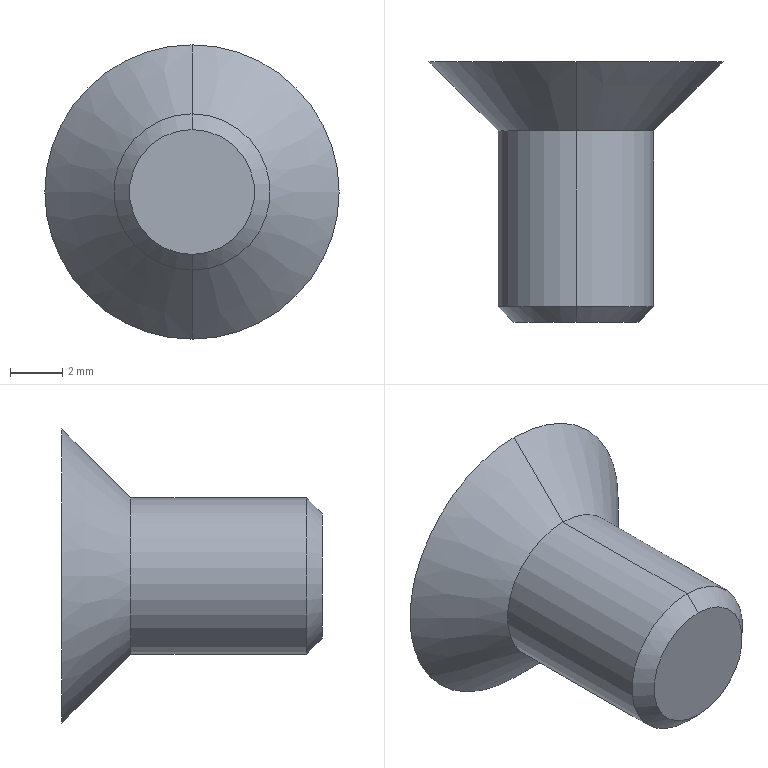Part | STEP file | 001-004-Hexagon socket countersunk head screw M6x10 | 1 solid | 21 faces | box 11.3 x 10 x 11.3 mm | volume 345.405 mm3 | plane 15 | cone 4 | cylinder 2 | commonest cylinder face diameters 6 x2
STEP:
#1=CARTESIAN_POINT('',(0.,0.,0.));
#2=DIRECTION('',(0.,0.,1.));
#3=DIRECTION('',(1.,0.,0.));
#4=AXIS2_PLACEMENT_3D('',#1,#2,#3);
#5=CARTESIAN_POINT('',(0.,-10.,-2.4));
#6=VERTEX_POINT('',#5);
#7=CARTESIAN_POINT('',(0.,-10.,2.4));
#8=VERTEX_POINT('',#7);
#9=CARTESIAN_POINT('',(0.,-10.,0.));
#10=DIRECTION('',(0.,-1.,0.));
#11=DIRECTION('',(0.,0.,-1.));
#12=AXIS2_PLACEMENT_3D('',#9,#10,#11);
#13=CIRCLE('',#12,2.4);
#14=CARTESIAN_POINT('',(0.,-10.,0.));
#15=DIRECTION('',(0.,1.,0.));
#16=DIRECTION('',(0.,0.,1.));
#17=AXIS2_PLACEMENT_3D('',#14,#15,#16);
#18=CONICAL_SURFACE('',#17,2.4,0.7854);
#19=CARTESIAN_POINT('',(3.142,0.));
#20=DIRECTION('',(-1.,0.));
#21=VECTOR('',#20,1.);
#22=LINE('',#19,#21);
#23=(GEOMETRIC_REPRESENTATION_CONTEXT(2)PARAMETRIC_REPRESENTATION_CONTEXT()REPRESENTATION_CONTEXT('',''));
#24=DEFINITIONAL_REPRESENTATION('',(#22),#23);
#25=PCURVE('',#18,#24);
#26=CARTESIAN_POINT('',(0.,-10.,0.));
#27=DIRECTION('',(0.,-1.,0.));
#28=DIRECTION('',(0.,0.,-1.));
#29=AXIS2_PLACEMENT_3D('',#26,#27,#28);
#30=PLANE('',#29);
#31=CARTESIAN_POINT('',(0.,0.));
#32=DIRECTION('',(1.,0.));
#33=AXIS2_PLACEMENT_2D('',#31,#32);
#34=CIRCLE('',#33,2.4);
#35=(GEOMETRIC_REPRESENTATION_CONTEXT(2)PARAMETRIC_REPRESENTATION_CONTEXT()REPRESENTATION_CONTEXT('',''));
#36=DEFINITIONAL_REPRESENTATION('',(#34),#35);
#37=PCURVE('',#30,#36);
#38=SURFACE_CURVE('',#13,(#25,#37),.PCURVE_S1.);
#39=EDGE_CURVE('',#6,#8,#38,.T.);
#40=ORIENTED_EDGE('',*,*,#39,.F.);
#41=CARTESIAN_POINT('',(0.,-9.4,-3.));
#42=VERTEX_POINT('',#41);
#43=CARTESIAN_POINT('',(0.,-10.,-2.4));
#44=DIRECTION('',(0.,0.7071,-0.7071));
#45=VECTOR('',#44,1.);
#46=LINE('',#43,#45);
#47=CARTESIAN_POINT('',(3.142,0.));
#48=DIRECTION('',(0.,1.));
#49=VECTOR('',#48,1.);
#50=LINE('',#47,#49);
#51=(GEOMETRIC_REPRESENTATION_CONTEXT(2)PARAMETRIC_REPRESENTATION_CONTEXT()REPRESENTATION_CONTEXT('',''));
#52=DEFINITIONAL_REPRESENTATION('',(#50),#51);
#53=PCURVE('',#18,#52);
#54=CARTESIAN_POINT('',(0.,-10.,0.));
#55=DIRECTION('',(0.,1.,0.));
#56=DIRECTION('',(0.,0.,1.));
#57=AXIS2_PLACEMENT_3D('',#54,#55,#56);
#58=CONICAL_SURFACE('',#57,2.4,0.7854);
#59=CARTESIAN_POINT('',(3.142,0.));
#60=DIRECTION('',(0.,1.));
#61=VECTOR('',#60,1.);
#62=LINE('',#59,#61);
#63=(GEOMETRIC_REPRESENTATION_CONTEXT(2)PARAMETRIC_REPRESENTATION_CONTEXT()REPRESENTATION_CONTEXT('',''));
#64=DEFINITIONAL_REPRESENTATION('',(#62),#63);
#65=PCURVE('',#58,#64);
#66=SURFACE_CURVE('',#46,(#53,#65),.PCURVE_S1.);
#67=EDGE_CURVE('',#6,#42,#66,.T.);
#68=ORIENTED_EDGE('',*,*,#67,.T.);
#69=CARTESIAN_POINT('',(0.,-9.4,3.));
#70=VERTEX_POINT('',#69);
#71=CARTESIAN_POINT('',(0.,-9.4,0.));
#72=DIRECTION('',(0.,1.,0.));
#73=DIRECTION('',(0.,0.,-1.));
#74=AXIS2_PLACEMENT_3D('',#71,#72,#73);
#75=CIRCLE('',#74,3.);
#76=CARTESIAN_POINT('',(-3.142,0.6));
#77=DIRECTION('',(1.,0.));
#78=VECTOR('',#77,1.);
#79=LINE('',#76,#78);
#80=(GEOMETRIC_REPRESENTATION_CONTEXT(2)PARAMETRIC_REPRESENTATION_CONTEXT()REPRESENTATION_CONTEXT('',''));
#81=DEFINITIONAL_REPRESENTATION('',(#79),#80);
#82=PCURVE('',#18,#81);
#83=CARTESIAN_POINT('',(0.,-10.,0.));
#84=DIRECTION('',(0.,1.,0.));
#85=DIRECTION('',(0.,0.,1.));
#86=AXIS2_PLACEMENT_3D('',#83,#84,#85);
#87=CYLINDRICAL_SURFACE('',#86,3.);
#88=CARTESIAN_POINT('',(-3.142,0.6));
#89=DIRECTION('',(1.,0.));
#90=VECTOR('',#89,1.);
#91=LINE('',#88,#90);
#92=(GEOMETRIC_REPRESENTATION_CONTEXT(2)PARAMETRIC_REPRESENTATION_CONTEXT()REPRESENTATION_CONTEXT('',''));
#93=DEFINITIONAL_REPRESENTATION('',(#91),#92);
#94=PCURVE('',#87,#93);
#95=SURFACE_CURVE('',#75,(#82,#94),.PCURVE_S1.);
#96=EDGE_CURVE('',#70,#42,#95,.T.);
#97=ORIENTED_EDGE('',*,*,#96,.F.);
#98=CARTESIAN_POINT('',(0.,-10.,2.4));
#99=DIRECTION('',(0.,0.7071,0.7071));
#100=VECTOR('',#99,1.);
#101=LINE('',#98,#100);
#102=CARTESIAN_POINT('',(0.,0.));
#103=DIRECTION('',(0.,1.));
#104=VECTOR('',#103,1.);
#105=LINE('',#102,#104);
#106=(GEOMETRIC_REPRESENTATION_CONTEXT(2)PARAMETRIC_REPRESENTATION_CONTEXT()REPRESENTATION_CONTEXT('',''));
#107=DEFINITIONAL_REPRESENTATION('',(#105),#106);
#108=PCURVE('',#18,#107);
#109=CARTESIAN_POINT('',(6.283,0.));
#110=DIRECTION('',(0.,1.));
#111=VECTOR('',#110,1.);
#112=LINE('',#109,#111);
#113=(GEOMETRIC_REPRESENTATION_CONTEXT(2)PARAMETRIC_REPRESENTATION_CONTEXT()REPRESENTATION_CONTEXT('',''));
#114=DEFINITIONAL_REPRESENTATION('',(#112),#113);
#115=PCURVE('',#58,#114);
#116=SURFACE_CURVE('',#101,(#108,#115),.PCURVE_S1.);
#117=EDGE_CURVE('',#8,#70,#116,.T.);
#118=ORIENTED_EDGE('',*,*,#117,.F.);
#119=EDGE_LOOP('',(#40,#68,#97,#118));
#120=FACE_BOUND('',#119,.T.);
#121=ADVANCED_FACE('',(#120),#18,.T.);
#122=ORIENTED_EDGE('',*,*,#96,.T.);
#123=CARTESIAN_POINT('',(0.,-2.65,-3.));
#124=VERTEX_POINT('',#123);
#125=CARTESIAN_POINT('',(0.,-10.,-3.));
#126=DIRECTION('',(0.,1.,0.));
#127=VECTOR('',#126,1.);
#128=LINE('',#125,#127);
#129=CARTESIAN_POINT('',(3.142,0.));
#130=DIRECTION('',(0.,1.));
#131=VECTOR('',#130,1.);
#132=LINE('',#129,#131);
#133=(GEOMETRIC_REPRESENTATION_CONTEXT(2)PARAMETRIC_REPRESENTATION_CONTEXT()REPRESENTATION_CONTEXT('',''));
#134=DEFINITIONAL_REPRESENTATION('',(#132),#133);
#135=PCURVE('',#87,#134);
#136=CARTESIAN_POINT('',(0.,-10.,0.));
#137=DIRECTION('',(0.,1.,0.));
#138=DIRECTION('',(0.,0.,1.));
#139=AXIS2_PLACEMENT_3D('',#136,#137,#138);
#140=CYLINDRICAL_SURFACE('',#139,3.);
#141=CARTESIAN_POINT('',(3.142,0.));
#142=DIRECTION('',(0.,1.));
#143=VECTOR('',#142,1.);
#144=LINE('',#141,#143);
#145=(GEOMETRIC_REPRESENTATION_CONTEXT(2)PARAMETRIC_REPRESENTATION_CONTEXT()REPRESENTATION_CONTEXT('',''));
#146=DEFINITIONAL_REPRESENTATION('',(#144),#145);
#147=PCURVE('',#140,#146);
#148=SURFACE_CURVE('',#128,(#135,#147),.PCURVE_S1.);
#149=EDGE_CURVE('',#42,#124,#148,.T.);
#150=ORIENTED_EDGE('',*,*,#149,.T.);
#151=CARTESIAN_POINT('',(0.,-2.65,3.));
#152=VERTEX_POINT('',#151);
#153=CARTESIAN_POINT('',(0.,-2.65,0.));
#154=DIRECTION('',(0.,1.,0.));
#155=DIRECTION('',(0.,0.,1.));
#156=AXIS2_PLACEMENT_3D('',#153,#154,#155);
#157=CIRCLE('',#156,3.);
#158=CARTESIAN_POINT('',(0.,7.35));
#159=DIRECTION('',(1.,0.));
#160=VECTOR('',#159,1.);
#161=LINE('',#158,#160);
#162=(GEOMETRIC_REPRESENTATION_CONTEXT(2)PARAMETRIC_REPRESENTATION_CONTEXT()REPRESENTATION_CONTEXT('',''));
#163=DEFINITIONAL_REPRESENTATION('',(#161),#162);
#164=PCURVE('',#87,#163);
#165=CARTESIAN_POINT('',(0.,-3.72,0.));
#166=DIRECTION('',(0.,1.,0.));
#167=DIRECTION('',(0.,0.,1.));
#168=AXIS2_PLACEMENT_3D('',#165,#166,#167);
#169=CONICAL_SURFACE('',#168,1.93,0.7854);
#170=CARTESIAN_POINT('',(0.,1.07));
#171=DIRECTION('',(1.,0.));
#172=VECTOR('',#171,1.);
#173=LINE('',#170,#172);
#174=(GEOMETRIC_REPRESENTATION_CONTEXT(2)PARAMETRIC_REPRESENTATION_CONTEXT()REPRESENTATION_CONTEXT('',''));
#175=DEFINITIONAL_REPRESENTATION('',(#173),#174);
#176=PCURVE('',#169,#175);
#177=SURFACE_CURVE('',#157,(#164,#176),.PCURVE_S1.);
#178=EDGE_CURVE('',#152,#124,#177,.T.);
#179=ORIENTED_EDGE('',*,*,#178,.F.);
#180=CARTESIAN_POINT('',(0.,-10.,3.));
#181=DIRECTION('',(0.,1.,0.));
#182=VECTOR('',#181,1.);
#183=LINE('',#180,#182);
#184=CARTESIAN_POINT('',(0.,0.));
#185=DIRECTION('',(0.,1.));
#186=VECTOR('',#185,1.);
#187=LINE('',#184,#186);
#188=(GEOMETRIC_REPRESENTATION_CONTEXT(2)PARAMETRIC_REPRESENTATION_CONTEXT()REPRESENTATION_CONTEXT('',''));
#189=DEFINITIONAL_REPRESENTATION('',(#187),#188);
#190=PCURVE('',#87,#189);
#191=CARTESIAN_POINT('',(6.283,0.));
#192=DIRECTION('',(0.,1.));
#193=VECTOR('',#192,1.);
#194=LINE('',#191,#193);
#195=(GEOMETRIC_REPRESENTATION_CONTEXT(2)PARAMETRIC_REPRESENTATION_CONTEXT()REPRESENTATION_CONTEXT('',''));
#196=DEFINITIONAL_REPRESENTATION('',(#194),#195);
#197=PCURVE('',#140,#196);
#198=SURFACE_CURVE('',#183,(#190,#197),.PCURVE_S1.);
#199=EDGE_CURVE('',#70,#152,#198,.T.);
#200=ORIENTED_EDGE('',*,*,#199,.F.);
#201=EDGE_LOOP('',(#122,#150,#179,#200));
#202=FACE_BOUND('',#201,.T.);
#203=ADVANCED_FACE('',(#202),#87,.T.);
#204=ORIENTED_EDGE('',*,*,#178,.T.);
#205=CARTESIAN_POINT('',(0.,0.,-5.65));
#206=VERTEX_POINT('',#205);
#207=CARTESIAN_POINT('',(0.,-3.72,-1.93));
#208=DIRECTION('',(0.,0.7071,-0.7071));
#209=VECTOR('',#208,1.);
#210=LINE('',#207,#209);
#211=CARTESIAN_POINT('',(3.142,0.));
#212=DIRECTION('',(0.,1.));
#213=VECTOR('',#212,1.);
#214=LINE('',#211,#213);
#215=(GEOMETRIC_REPRESENTATION_CONTEXT(2)PARAMETRIC_REPRESENTATION_CONTEXT()REPRESENTATION_CONTEXT('',''));
#216=DEFINITIONAL_REPRESENTATION('',(#214),#215);
#217=PCURVE('',#169,#216);
#218=CARTESIAN_POINT('',(0.,-3.72,0.));
#219=DIRECTION('',(0.,1.,0.));
#220=DIRECTION('',(0.,0.,1.));
#221=AXIS2_PLACEMENT_3D('',#218,#219,#220);
#222=CONICAL_SURFACE('',#221,1.93,0.7854);
#223=CARTESIAN_POINT('',(3.142,0.));
#224=DIRECTION('',(0.,1.));
#225=VECTOR('',#224,1.);
#226=LINE('',#223,#225);
#227=(GEOMETRIC_REPRESENTATION_CONTEXT(2)PARAMETRIC_REPRESENTATION_CONTEXT()REPRESENTATION_CONTEXT('',''));
#228=DEFINITIONAL_REPRESENTATION('',(#226),#227);
#229=PCURVE('',#222,#228);
#230=SURFACE_CURVE('',#210,(#217,#229),.PCURVE_S1.);
#231=EDGE_CURVE('',#124,#206,#230,.T.);
#232=ORIENTED_EDGE('',*,*,#231,.T.);
#233=CARTESIAN_POINT('',(0.,0.,5.65));
#234=VERTEX_POINT('',#233);
#235=CARTESIAN_POINT('',(0.,0.,0.));
#236=DIRECTION('',(0.,-1.,0.));
#237=DIRECTION('',(0.,0.,-1.));
#238=AXIS2_PLACEMENT_3D('',#235,#236,#237);
#239=CIRCLE('',#238,5.65);
#240=CARTESIAN_POINT('',(3.142,3.72));
#241=DIRECTION('',(-1.,0.));
#242=VECTOR('',#241,1.);
#243=LINE('',#240,#242);
#244=(GEOMETRIC_REPRESENTATION_CONTEXT(2)PARAMETRIC_REPRESENTATION_CONTEXT()REPRESENTATION_CONTEXT('',''));
#245=DEFINITIONAL_REPRESENTATION('',(#243),#244);
#246=PCURVE('',#169,#245);
#247=CARTESIAN_POINT('',(0.,0.,0.));
#248=DIRECTION('',(0.,1.,0.));
#249=DIRECTION('',(0.,0.,1.));
#250=AXIS2_PLACEMENT_3D('',#247,#248,#249);
#251=PLANE('',#250);
#252=CARTESIAN_POINT('',(-5.65,0.));
#253=CARTESIAN_POINT('',(-5.65,9.786));
#254=CARTESIAN_POINT('',(2.825,4.893));
#255=CARTESIAN_POINT('',(11.3,0.));
#256=CARTESIAN_POINT('',(2.825,-4.893));
#257=CARTESIAN_POINT('',(-5.65,-9.786));
#258=CARTESIAN_POINT('',(-5.65,0.));
#259=(BOUNDED_CURVE()B_SPLINE_CURVE(2,(#252,#253,#254,#255,#256,#257,#258),.UNSPECIFIED.,.T.,.F.)B_SPLINE_CURVE_WITH_KNOTS((1,2,2,2,2,1),(-2.094,0.,2.094,4.189,6.283,8.378),.UNSPECIFIED.)CURVE()GEOMETRIC_REPRESENTATION_ITEM()RATIONAL_B_SPLINE_CURVE((1.,0.5,1.,0.5,1.,0.5,1.))REPRESENTATION_ITEM(''));
#260=(GEOMETRIC_REPRESENTATION_CONTEXT(2)PARAMETRIC_REPRESENTATION_CONTEXT()REPRESENTATION_CONTEXT('',''));
#261=DEFINITIONAL_REPRESENTATION('',(#259),#260);
#262=PCURVE('',#251,#261);
#263=SURFACE_CURVE('',#239,(#246,#262),.PCURVE_S1.);
#264=EDGE_CURVE('',#206,#234,#263,.T.);
#265=ORIENTED_EDGE('',*,*,#264,.T.);
#266=CARTESIAN_POINT('',(0.,-3.72,1.93));
#267=DIRECTION('',(0.,0.7071,0.7071));
#268=VECTOR('',#267,1.);
#269=LINE('',#266,#268);
#270=CARTESIAN_POINT('',(0.,0.));
#271=DIRECTION('',(0.,1.));
#272=VECTOR('',#271,1.);
#273=LINE('',#270,#272);
#274=(GEOMETRIC_REPRESENTATION_CONTEXT(2)PARAMETRIC_REPRESENTATION_CONTEXT()REPRESENTATION_CONTEXT('',''));
#275=DEFINITIONAL_REPRESENTATION('',(#273),#274);
#276=PCURVE('',#169,#275);
#277=CARTESIAN_POINT('',(6.283,0.));
#278=DIRECTION('',(0.,1.));
#279=VECTOR('',#278,1.);
#280=LINE('',#277,#279);
#281=(GEOMETRIC_REPRESENTATION_CONTEXT(2)PARAMETRIC_REPRESENTATION_CONTEXT()REPRESENTATION_CONTEXT('',''));
#282=DEFINITIONAL_REPRESENTATION('',(#280),#281);
#283=PCURVE('',#222,#282);
#284=SURFACE_CURVE('',#269,(#276,#283),.PCURVE_S1.);
#285=EDGE_CURVE('',#152,#234,#284,.T.);
#286=ORIENTED_EDGE('',*,*,#285,.F.);
#287=EDGE_LOOP('',(#204,#232,#265,#286));
#288=FACE_BOUND('',#287,.T.);
#289=ADVANCED_FACE('',(#288),#169,.T.);
#290=ORIENTED_EDGE('',*,*,#231,.F.);
#291=CARTESIAN_POINT('',(0.,-2.65,0.));
#292=DIRECTION('',(0.,1.,0.));
#293=DIRECTION('',(0.,0.,1.));
#294=AXIS2_PLACEMENT_3D('',#291,#292,#293);
#295=CIRCLE('',#294,3.);
#296=CARTESIAN_POINT('',(0.,1.07));
#297=DIRECTION('',(1.,0.));
#298=VECTOR('',#297,1.);
#299=LINE('',#296,#298);
#300=(GEOMETRIC_REPRESENTATION_CONTEXT(2)PARAMETRIC_REPRESENTATION_CONTEXT()REPRESENTATION_CONTEXT('',''));
#301=DEFINITIONAL_REPRESENTATION('',(#299),#300);
#302=PCURVE('',#222,#301);
#303=CARTESIAN_POINT('',(0.,7.35));
#304=DIRECTION('',(1.,0.));
#305=VECTOR('',#304,1.);
#306=LINE('',#303,#305);
#307=(GEOMETRIC_REPRESENTATION_CONTEXT(2)PARAMETRIC_REPRESENTATION_CONTEXT()REPRESENTATION_CONTEXT('',''));
#308=DEFINITIONAL_REPRESENTATION('',(#306),#307);
#309=PCURVE('',#140,#308);
#310=SURFACE_CURVE('',#295,(#302,#309),.PCURVE_S1.);
#311=EDGE_CURVE('',#124,#152,#310,.T.);
#312=ORIENTED_EDGE('',*,*,#311,.T.);
#313=ORIENTED_EDGE('',*,*,#285,.T.);
#314=CARTESIAN_POINT('',(0.,0.,0.));
#315=DIRECTION('',(0.,-1.,0.));
#316=DIRECTION('',(0.,0.,-1.));
#317=AXIS2_PLACEMENT_3D('',#314,#315,#316);
#318=CIRCLE('',#317,5.65);
#319=CARTESIAN_POINT('',(9.425,3.72));
#320=DIRECTION('',(-1.,0.));
#321=VECTOR('',#320,1.);
#322=LINE('',#319,#321);
#323=(GEOMETRIC_REPRESENTATION_CONTEXT(2)PARAMETRIC_REPRESENTATION_CONTEXT()REPRESENTATION_CONTEXT('',''));
#324=DEFINITIONAL_REPRESENTATION('',(#322),#323);
#325=PCURVE('',#222,#324);
#326=CARTESIAN_POINT('',(-5.65,0.));
#327=CARTESIAN_POINT('',(-5.65,9.786));
#328=CARTESIAN_POINT('',(2.825,4.893));
#329=CARTESIAN_POINT('',(11.3,0.));
#330=CARTESIAN_POINT('',(2.825,-4.893));
#331=CARTESIAN_POINT('',(-5.65,-9.786));
#332=CARTESIAN_POINT('',(-5.65,0.));
#333=(BOUNDED_CURVE()B_SPLINE_CURVE(2,(#326,#327,#328,#329,#330,#331,#332),.UNSPECIFIED.,.T.,.F.)B_SPLINE_CURVE_WITH_KNOTS((1,2,2,2,2,1),(-2.094,0.,2.094,4.189,6.283,8.378),.UNSPECIFIED.)CURVE()GEOMETRIC_REPRESENTATION_ITEM()RATIONAL_B_SPLINE_CURVE((1.,0.5,1.,0.5,1.,0.5,1.))REPRESENTATION_ITEM(''));
#334=(GEOMETRIC_REPRESENTATION_CONTEXT(2)PARAMETRIC_REPRESENTATION_CONTEXT()REPRESENTATION_CONTEXT('',''));
#335=DEFINITIONAL_REPRESENTATION('',(#333),#334);
#336=PCURVE('',#251,#335);
#337=SURFACE_CURVE('',#318,(#325,#336),.PCURVE_S1.);
#338=EDGE_CURVE('',#234,#206,#337,.T.);
#339=ORIENTED_EDGE('',*,*,#338,.T.);
#340=EDGE_LOOP('',(#290,#312,#313,#339));
#341=FACE_BOUND('',#340,.T.);
#342=ADVANCED_FACE('',(#341),#222,.T.);
#343=CARTESIAN_POINT('',(2.,0.,1.155));
#344=VERTEX_POINT('',#343);
#345=CARTESIAN_POINT('',(2.,0.,-1.155));
#346=VERTEX_POINT('',#345);
#347=CARTESIAN_POINT('',(2.,0.,1.155));
#348=DIRECTION('',(0.,0.,-1.));
#349=VECTOR('',#348,1.);
#350=LINE('',#347,#349);
#351=CARTESIAN_POINT('',(1.155,2.));
#352=DIRECTION('',(-1.,0.));
#353=VECTOR('',#352,1.);
#354=LINE('',#351,#353);
#355=(GEOMETRIC_REPRESENTATION_CONTEXT(2)PARAMETRIC_REPRESENTATION_CONTEXT()REPRESENTATION_CONTEXT('',''));
#356=DEFINITIONAL_REPRESENTATION('',(#354),#355);
#357=PCURVE('',#251,#356);
#358=CARTESIAN_POINT('',(2.,-2.2,1.155));
#359=DIRECTION('',(1.,0.,0.));
#360=DIRECTION('',(0.,0.,-1.));
#361=AXIS2_PLACEMENT_3D('',#358,#359,#360);
#362=PLANE('',#361);
#363=CARTESIAN_POINT('',(0.,2.2));
#364=DIRECTION('',(1.,0.));
#365=VECTOR('',#364,1.);
#366=LINE('',#363,#365);
#367=(GEOMETRIC_REPRESENTATION_CONTEXT(2)PARAMETRIC_REPRESENTATION_CONTEXT()REPRESENTATION_CONTEXT('',''));
#368=DEFINITIONAL_REPRESENTATION('',(#366),#367);
#369=PCURVE('',#362,#368);
#370=SURFACE_CURVE('',#350,(#357,#369),.PCURVE_S1.);
#371=EDGE_CURVE('',#344,#346,#370,.T.);
#372=ORIENTED_EDGE('',*,*,#371,.F.);
#373=CARTESIAN_POINT('',(0.,0.,2.309));
#374=VERTEX_POINT('',#373);
#375=CARTESIAN_POINT('',(0.,0.,2.309));
#376=DIRECTION('',(0.866,0.,-0.5));
#377=VECTOR('',#376,1.);
#378=LINE('',#375,#377);
#379=CARTESIAN_POINT('',(2.309,0.));
#380=DIRECTION('',(-0.5,0.866));
#381=VECTOR('',#380,1.);
#382=LINE('',#379,#381);
#383=(GEOMETRIC_REPRESENTATION_CONTEXT(2)PARAMETRIC_REPRESENTATION_CONTEXT()REPRESENTATION_CONTEXT('',''));
#384=DEFINITIONAL_REPRESENTATION('',(#382),#383);
#385=PCURVE('',#251,#384);
#386=CARTESIAN_POINT('',(0.,-2.2,2.309));
#387=DIRECTION('',(0.5,0.,0.866));
#388=DIRECTION('',(0.866,0.,-0.5));
#389=AXIS2_PLACEMENT_3D('',#386,#387,#388);
#390=PLANE('',#389);
#391=CARTESIAN_POINT('',(0.,2.2));
#392=DIRECTION('',(1.,0.));
#393=VECTOR('',#392,1.);
#394=LINE('',#391,#393);
#395=(GEOMETRIC_REPRESENTATION_CONTEXT(2)PARAMETRIC_REPRESENTATION_CONTEXT()REPRESENTATION_CONTEXT('',''));
#396=DEFINITIONAL_REPRESENTATION('',(#394),#395);
#397=PCURVE('',#390,#396);
#398=SURFACE_CURVE('',#378,(#385,#397),.PCURVE_S1.);
#399=EDGE_CURVE('',#374,#344,#398,.T.);
#400=ORIENTED_EDGE('',*,*,#399,.F.);
#401=CARTESIAN_POINT('',(-2.,0.,1.155));
#402=VERTEX_POINT('',#401);
#403=CARTESIAN_POINT('',(-2.,0.,1.155));
#404=DIRECTION('',(0.866,0.,0.5));
#405=VECTOR('',#404,1.);
#406=LINE('',#403,#405);
#407=CARTESIAN_POINT('',(1.155,-2.));
#408=DIRECTION('',(0.5,0.866));
#409=VECTOR('',#408,1.);
#410=LINE('',#407,#409);
#411=(GEOMETRIC_REPRESENTATION_CONTEXT(2)PARAMETRIC_REPRESENTATION_CONTEXT()REPRESENTATION_CONTEXT('',''));
#412=DEFINITIONAL_REPRESENTATION('',(#410),#411);
#413=PCURVE('',#251,#412);
#414=CARTESIAN_POINT('',(-2.,-2.2,1.155));
#415=DIRECTION('',(-0.5,0.,0.866));
#416=DIRECTION('',(0.866,0.,0.5));
#417=AXIS2_PLACEMENT_3D('',#414,#415,#416);
#418=PLANE('',#417);
#419=CARTESIAN_POINT('',(0.,2.2));
#420=DIRECTION('',(1.,0.));
#421=VECTOR('',#420,1.);
#422=LINE('',#419,#421);
#423=(GEOMETRIC_REPRESENTATION_CONTEXT(2)PARAMETRIC_REPRESENTATION_CONTEXT()REPRESENTATION_CONTEXT('',''));
#424=DEFINITIONAL_REPRESENTATION('',(#422),#423);
#425=PCURVE('',#418,#424);
#426=SURFACE_CURVE('',#406,(#413,#425),.PCURVE_S1.);
#427=EDGE_CURVE('',#402,#374,#426,.T.);
#428=ORIENTED_EDGE('',*,*,#427,.F.);
#429=CARTESIAN_POINT('',(-2.,0.,-1.155));
#430=VERTEX_POINT('',#429);
#431=CARTESIAN_POINT('',(-2.,0.,-1.155));
#432=DIRECTION('',(0.,0.,1.));
#433=VECTOR('',#432,1.);
#434=LINE('',#431,#433);
#435=CARTESIAN_POINT('',(-1.155,-2.));
#436=DIRECTION('',(1.,0.));
#437=VECTOR('',#436,1.);
#438=LINE('',#435,#437);
#439=(GEOMETRIC_REPRESENTATION_CONTEXT(2)PARAMETRIC_REPRESENTATION_CONTEXT()REPRESENTATION_CONTEXT('',''));
#440=DEFINITIONAL_REPRESENTATION('',(#438),#439);
#441=PCURVE('',#251,#440);
#442=CARTESIAN_POINT('',(-2.,-2.2,-1.155));
#443=DIRECTION('',(-1.,0.,0.));
#444=DIRECTION('',(0.,0.,1.));
#445=AXIS2_PLACEMENT_3D('',#442,#443,#444);
#446=PLANE('',#445);
#447=CARTESIAN_POINT('',(0.,2.2));
#448=DIRECTION('',(1.,0.));
#449=VECTOR('',#448,1.);
#450=LINE('',#447,#449);
#451=(GEOMETRIC_REPRESENTATION_CONTEXT(2)PARAMETRIC_REPRESENTATION_CONTEXT()REPRESENTATION_CONTEXT('',''));
#452=DEFINITIONAL_REPRESENTATION('',(#450),#451);
#453=PCURVE('',#446,#452);
#454=SURFACE_CURVE('',#434,(#441,#453),.PCURVE_S1.);
#455=EDGE_CURVE('',#430,#402,#454,.T.);
#456=ORIENTED_EDGE('',*,*,#455,.F.);
#457=CARTESIAN_POINT('',(0.,0.,-2.309));
#458=VERTEX_POINT('',#457);
#459=CARTESIAN_POINT('',(0.,0.,-2.309));
#460=DIRECTION('',(-0.866,0.,0.5));
#461=VECTOR('',#460,1.);
#462=LINE('',#459,#461);
#463=CARTESIAN_POINT('',(-2.309,0.));
#464=DIRECTION('',(0.5,-0.866));
#465=VECTOR('',#464,1.);
#466=LINE('',#463,#465);
#467=(GEOMETRIC_REPRESENTATION_CONTEXT(2)PARAMETRIC_REPRESENTATION_CONTEXT()REPRESENTATION_CONTEXT('',''));
#468=DEFINITIONAL_REPRESENTATION('',(#466),#467);
#469=PCURVE('',#251,#468);
#470=CARTESIAN_POINT('',(0.,-2.2,-2.309));
#471=DIRECTION('',(-0.5,0.,-0.866));
#472=DIRECTION('',(-0.866,0.,0.5));
#473=AXIS2_PLACEMENT_3D('',#470,#471,#472);
#474=PLANE('',#473);
#475=CARTESIAN_POINT('',(0.,2.2));
#476=DIRECTION('',(1.,0.));
#477=VECTOR('',#476,1.);
#478=LINE('',#475,#477);
#479=(GEOMETRIC_REPRESENTATION_CONTEXT(2)PARAMETRIC_REPRESENTATION_CONTEXT()REPRESENTATION_CONTEXT('',''));
#480=DEFINITIONAL_REPRESENTATION('',(#478),#479);
#481=PCURVE('',#474,#480);
#482=SURFACE_CURVE('',#462,(#469,#481),.PCURVE_S1.);
#483=EDGE_CURVE('',#458,#430,#482,.T.);
#484=ORIENTED_EDGE('',*,*,#483,.F.);
#485=CARTESIAN_POINT('',(2.,0.,-1.155));
#486=DIRECTION('',(-0.866,0.,-0.5));
#487=VECTOR('',#486,1.);
#488=LINE('',#485,#487);
#489=CARTESIAN_POINT('',(-1.155,2.));
#490=DIRECTION('',(-0.5,-0.866));
#491=VECTOR('',#490,1.);
#492=LINE('',#489,#491);
#493=(GEOMETRIC_REPRESENTATION_CONTEXT(2)PARAMETRIC_REPRESENTATION_CONTEXT()REPRESENTATION_CONTEXT('',''));
#494=DEFINITIONAL_REPRESENTATION('',(#492),#493);
#495=PCURVE('',#251,#494);
#496=CARTESIAN_POINT('',(2.,-2.2,-1.155));
#497=DIRECTION('',(0.5,0.,-0.866));
#498=DIRECTION('',(-0.866,0.,-0.5));
#499=AXIS2_PLACEMENT_3D('',#496,#497,#498);
#500=PLANE('',#499);
#501=CARTESIAN_POINT('',(0.,2.2));
#502=DIRECTION('',(1.,0.));
#503=VECTOR('',#502,1.);
#504=LINE('',#501,#503);
#505=(GEOMETRIC_REPRESENTATION_CONTEXT(2)PARAMETRIC_REPRESENTATION_CONTEXT()REPRESENTATION_CONTEXT('',''));
#506=DEFINITIONAL_REPRESENTATION('',(#504),#505);
#507=PCURVE('',#500,#506);
#508=SURFACE_CURVE('',#488,(#495,#507),.PCURVE_S1.);
#509=EDGE_CURVE('',#346,#458,#508,.T.);
#510=ORIENTED_EDGE('',*,*,#509,.F.);
#511=EDGE_LOOP('',(#372,#400,#428,#456,#484,#510));
#512=FACE_BOUND('',#511,.T.);
#513=ORIENTED_EDGE('',*,*,#338,.F.);
#514=ORIENTED_EDGE('',*,*,#264,.F.);
#515=EDGE_LOOP('',(#513,#514));
#516=FACE_BOUND('',#515,.T.);
#517=ADVANCED_FACE('',(#512,#516),#251,.T.);
#518=ORIENTED_EDGE('',*,*,#149,.F.);
#519=CARTESIAN_POINT('',(0.,-9.4,0.));
#520=DIRECTION('',(0.,1.,0.));
#521=DIRECTION('',(0.,0.,-1.));
#522=AXIS2_PLACEMENT_3D('',#519,#520,#521);
#523=CIRCLE('',#522,3.);
#524=CARTESIAN_POINT('',(3.142,0.6));
#525=DIRECTION('',(1.,0.));
#526=VECTOR('',#525,1.);
#527=LINE('',#524,#526);
#528=(GEOMETRIC_REPRESENTATION_CONTEXT(2)PARAMETRIC_REPRESENTATION_CONTEXT()REPRESENTATION_CONTEXT('',''));
#529=DEFINITIONAL_REPRESENTATION('',(#527),#528);
#530=PCURVE('',#140,#529);
#531=CARTESIAN_POINT('',(3.142,0.6));
#532=DIRECTION('',(1.,0.));
#533=VECTOR('',#532,1.);
#534=LINE('',#531,#533);
#535=(GEOMETRIC_REPRESENTATION_CONTEXT(2)PARAMETRIC_REPRESENTATION_CONTEXT()REPRESENTATION_CONTEXT('',''));
#536=DEFINITIONAL_REPRESENTATION('',(#534),#535);
#537=PCURVE('',#58,#536);
#538=SURFACE_CURVE('',#523,(#530,#537),.PCURVE_S1.);
#539=EDGE_CURVE('',#42,#70,#538,.T.);
#540=ORIENTED_EDGE('',*,*,#539,.T.);
#541=ORIENTED_EDGE('',*,*,#199,.T.);
#542=ORIENTED_EDGE('',*,*,#311,.F.);
#543=EDGE_LOOP('',(#518,#540,#541,#542));
#544=FACE_BOUND('',#543,.T.);
#545=ADVANCED_FACE('',(#544),#140,.T.);
#546=CARTESIAN_POINT('',(0.,-10.,0.));
#547=DIRECTION('',(0.,-1.,0.));
#548=DIRECTION('',(0.,0.,-1.));
#549=AXIS2_PLACEMENT_3D('',#546,#547,#548);
#550=CIRCLE('',#549,2.4);
#551=CARTESIAN_POINT('',(0.,0.));
#552=DIRECTION('',(1.,0.));
#553=AXIS2_PLACEMENT_2D('',#551,#552);
#554=CIRCLE('',#553,2.4);
#555=(GEOMETRIC_REPRESENTATION_CONTEXT(2)PARAMETRIC_REPRESENTATION_CONTEXT()REPRESENTATION_CONTEXT('',''));
#556=DEFINITIONAL_REPRESENTATION('',(#554),#555);
#557=PCURVE('',#30,#556);
#558=CARTESIAN_POINT('',(9.425,0.));
#559=DIRECTION('',(-1.,0.));
#560=VECTOR('',#559,1.);
#561=LINE('',#558,#560);
#562=(GEOMETRIC_REPRESENTATION_CONTEXT(2)PARAMETRIC_REPRESENTATION_CONTEXT()REPRESENTATION_CONTEXT('',''));
#563=DEFINITIONAL_REPRESENTATION('',(#561),#562);
#564=PCURVE('',#58,#563);
#565=SURFACE_CURVE('',#550,(#557,#564),.PCURVE_S1.);
#566=EDGE_CURVE('',#8,#6,#565,.T.);
#567=ORIENTED_EDGE('',*,*,#566,.T.);
#568=ORIENTED_EDGE('',*,*,#39,.T.);
#569=EDGE_LOOP('',(#567,#568));
#570=FACE_BOUND('',#569,.T.);
#571=ADVANCED_FACE('',(#570),#30,.T.);
#572=CARTESIAN_POINT('',(2.,-1.047,-1.155));
#573=VERTEX_POINT('',#572);
#574=CARTESIAN_POINT('',(2.,-2.2,-1.155));
#575=DIRECTION('',(0.,1.,0.));
#576=VECTOR('',#575,1.);
#577=LINE('',#574,#576);
#578=CARTESIAN_POINT('',(2.309,0.));
#579=DIRECTION('',(0.,1.));
#580=VECTOR('',#579,1.);
#581=LINE('',#578,#580);
#582=(GEOMETRIC_REPRESENTATION_CONTEXT(2)PARAMETRIC_REPRESENTATION_CONTEXT()REPRESENTATION_CONTEXT('',''));
#583=DEFINITIONAL_REPRESENTATION('',(#581),#582);
#584=PCURVE('',#362,#583);
#585=CARTESIAN_POINT('',(0.,0.));
#586=DIRECTION('',(0.,1.));
#587=VECTOR('',#586,1.);
#588=LINE('',#585,#587);
#589=(GEOMETRIC_REPRESENTATION_CONTEXT(2)PARAMETRIC_REPRESENTATION_CONTEXT()REPRESENTATION_CONTEXT('',''));
#590=DEFINITIONAL_REPRESENTATION('',(#588),#589);
#591=PCURVE('',#500,#590);
#592=SURFACE_CURVE('',#577,(#584,#591),.PCURVE_S1.);
#593=EDGE_CURVE('',#573,#346,#592,.T.);
#594=ORIENTED_EDGE('',*,*,#593,.F.);
#595=CARTESIAN_POINT('',(2.,-1.047,1.155));
#596=VERTEX_POINT('',#595);
#597=CARTESIAN_POINT('',(2.,-1.047,1.155));
#598=DIRECTION('',(0.,0.,1.));
#599=VECTOR('',#598,1.);
#600=LINE('',#597,#599);
#601=CARTESIAN_POINT('',(0.,1.153));
#602=DIRECTION('',(-1.,0.));
#603=VECTOR('',#602,1.);
#604=LINE('',#601,#603);
#605=(GEOMETRIC_REPRESENTATION_CONTEXT(2)PARAMETRIC_REPRESENTATION_CONTEXT()REPRESENTATION_CONTEXT('',''));
#606=DEFINITIONAL_REPRESENTATION('',(#604),#605);
#607=PCURVE('',#362,#606);
#608=CARTESIAN_POINT('',(0.0034,-2.2,0.));
#609=DIRECTION('',(0.5,-0.866,0.));
#610=DIRECTION('',(0.,0.,-1.));
#611=AXIS2_PLACEMENT_3D('',#608,#609,#610);
#612=PLANE('',#611);
#613=CARTESIAN_POINT('',(-1.155,2.305));
#614=DIRECTION('',(-1.,0.));
#615=VECTOR('',#614,1.);
#616=LINE('',#613,#615);
#617=(GEOMETRIC_REPRESENTATION_CONTEXT(2)PARAMETRIC_REPRESENTATION_CONTEXT()REPRESENTATION_CONTEXT('',''));
#618=DEFINITIONAL_REPRESENTATION('',(#616),#617);
#619=PCURVE('',#612,#618);
#620=SURFACE_CURVE('',#600,(#607,#619),.PCURVE_S1.);
#621=EDGE_CURVE('',#573,#596,#620,.T.);
#622=ORIENTED_EDGE('',*,*,#621,.T.);
#623=CARTESIAN_POINT('',(2.,-2.2,1.155));
#624=DIRECTION('',(0.,1.,0.));
#625=VECTOR('',#624,1.);
#626=LINE('',#623,#625);
#627=CARTESIAN_POINT('',(0.,0.));
#628=DIRECTION('',(0.,1.));
#629=VECTOR('',#628,1.);
#630=LINE('',#627,#629);
#631=(GEOMETRIC_REPRESENTATION_CONTEXT(2)PARAMETRIC_REPRESENTATION_CONTEXT()REPRESENTATION_CONTEXT('',''));
#632=DEFINITIONAL_REPRESENTATION('',(#630),#631);
#633=PCURVE('',#362,#632);
#634=CARTESIAN_POINT('',(2.309,0.));
#635=DIRECTION('',(0.,1.));
#636=VECTOR('',#635,1.);
#637=LINE('',#634,#636);
#638=(GEOMETRIC_REPRESENTATION_CONTEXT(2)PARAMETRIC_REPRESENTATION_CONTEXT()REPRESENTATION_CONTEXT('',''));
#639=DEFINITIONAL_REPRESENTATION('',(#637),#638);
#640=PCURVE('',#390,#639);
#641=SURFACE_CURVE('',#626,(#633,#640),.PCURVE_S1.);
#642=EDGE_CURVE('',#596,#344,#641,.T.);
#643=ORIENTED_EDGE('',*,*,#642,.T.);
#644=ORIENTED_EDGE('',*,*,#371,.T.);
#645=EDGE_LOOP('',(#594,#622,#643,#644));
#646=FACE_BOUND('',#645,.T.);
#647=ADVANCED_FACE('',(#646),#362,.F.);
#648=ORIENTED_EDGE('',*,*,#642,.F.);
#649=CARTESIAN_POINT('',(0.,-1.047,2.309));
#650=VERTEX_POINT('',#649);
#651=CARTESIAN_POINT('',(0.,-1.047,2.309));
#652=DIRECTION('',(-0.866,0.,0.5));
#653=VECTOR('',#652,1.);
#654=LINE('',#651,#653);
#655=CARTESIAN_POINT('',(0.,1.153));
#656=DIRECTION('',(-1.,0.));
#657=VECTOR('',#656,1.);
#658=LINE('',#655,#657);
#659=(GEOMETRIC_REPRESENTATION_CONTEXT(2)PARAMETRIC_REPRESENTATION_CONTEXT()REPRESENTATION_CONTEXT('',''));
#660=DEFINITIONAL_REPRESENTATION('',(#658),#659);
#661=PCURVE('',#390,#660);
#662=CARTESIAN_POINT('',(0.0017,-2.2,0.002944));
#663=DIRECTION('',(0.25,-0.866,0.433));
#664=DIRECTION('',(0.866,0.,-0.5));
#665=AXIS2_PLACEMENT_3D('',#662,#663,#664);
#666=PLANE('',#665);
#667=CARTESIAN_POINT('',(-1.155,2.305));
#668=DIRECTION('',(-1.,0.));
#669=VECTOR('',#668,1.);
#670=LINE('',#667,#669);
#671=(GEOMETRIC_REPRESENTATION_CONTEXT(2)PARAMETRIC_REPRESENTATION_CONTEXT()REPRESENTATION_CONTEXT('',''));
#672=DEFINITIONAL_REPRESENTATION('',(#670),#671);
#673=PCURVE('',#666,#672);
#674=SURFACE_CURVE('',#654,(#661,#673),.PCURVE_S1.);
#675=EDGE_CURVE('',#596,#650,#674,.T.);
#676=ORIENTED_EDGE('',*,*,#675,.T.);
#677=CARTESIAN_POINT('',(0.,-2.2,2.309));
#678=DIRECTION('',(0.,1.,0.));
#679=VECTOR('',#678,1.);
#680=LINE('',#677,#679);
#681=CARTESIAN_POINT('',(0.,0.));
#682=DIRECTION('',(0.,1.));
#683=VECTOR('',#682,1.);
#684=LINE('',#681,#683);
#685=(GEOMETRIC_REPRESENTATION_CONTEXT(2)PARAMETRIC_REPRESENTATION_CONTEXT()REPRESENTATION_CONTEXT('',''));
#686=DEFINITIONAL_REPRESENTATION('',(#684),#685);
#687=PCURVE('',#390,#686);
#688=CARTESIAN_POINT('',(2.309,0.));
#689=DIRECTION('',(0.,1.));
#690=VECTOR('',#689,1.);
#691=LINE('',#688,#690);
#692=(GEOMETRIC_REPRESENTATION_CONTEXT(2)PARAMETRIC_REPRESENTATION_CONTEXT()REPRESENTATION_CONTEXT('',''));
#693=DEFINITIONAL_REPRESENTATION('',(#691),#692);
#694=PCURVE('',#418,#693);
#695=SURFACE_CURVE('',#680,(#687,#694),.PCURVE_S1.);
#696=EDGE_CURVE('',#650,#374,#695,.T.);
#697=ORIENTED_EDGE('',*,*,#696,.T.);
#698=ORIENTED_EDGE('',*,*,#399,.T.);
#699=EDGE_LOOP('',(#648,#676,#697,#698));
#700=FACE_BOUND('',#699,.T.);
#701=ADVANCED_FACE('',(#700),#390,.F.);
#702=ORIENTED_EDGE('',*,*,#696,.F.);
#703=CARTESIAN_POINT('',(-2.,-1.047,1.155));
#704=VERTEX_POINT('',#703);
#705=CARTESIAN_POINT('',(-2.,-1.047,1.155));
#706=DIRECTION('',(-0.866,0.,-0.5));
#707=VECTOR('',#706,1.);
#708=LINE('',#705,#707);
#709=CARTESIAN_POINT('',(0.,1.153));
#710=DIRECTION('',(-1.,0.));
#711=VECTOR('',#710,1.);
#712=LINE('',#709,#711);
#713=(GEOMETRIC_REPRESENTATION_CONTEXT(2)PARAMETRIC_REPRESENTATION_CONTEXT()REPRESENTATION_CONTEXT('',''));
#714=DEFINITIONAL_REPRESENTATION('',(#712),#713);
#715=PCURVE('',#418,#714);
#716=CARTESIAN_POINT('',(-0.0017,-2.2,0.002944));
#717=DIRECTION('',(-0.25,-0.866,0.433));
#718=DIRECTION('',(0.866,0.,0.5));
#719=AXIS2_PLACEMENT_3D('',#716,#717,#718);
#720=PLANE('',#719);
#721=CARTESIAN_POINT('',(-1.155,2.305));
#722=DIRECTION('',(-1.,0.));
#723=VECTOR('',#722,1.);
#724=LINE('',#721,#723);
#725=(GEOMETRIC_REPRESENTATION_CONTEXT(2)PARAMETRIC_REPRESENTATION_CONTEXT()REPRESENTATION_CONTEXT('',''));
#726=DEFINITIONAL_REPRESENTATION('',(#724),#725);
#727=PCURVE('',#720,#726);
#728=SURFACE_CURVE('',#708,(#715,#727),.PCURVE_S1.);
#729=EDGE_CURVE('',#650,#704,#728,.T.);
#730=ORIENTED_EDGE('',*,*,#729,.T.);
#731=CARTESIAN_POINT('',(-2.,-2.2,1.155));
#732=DIRECTION('',(0.,1.,0.));
#733=VECTOR('',#732,1.);
#734=LINE('',#731,#733);
#735=CARTESIAN_POINT('',(0.,0.));
#736=DIRECTION('',(0.,1.));
#737=VECTOR('',#736,1.);
#738=LINE('',#735,#737);
#739=(GEOMETRIC_REPRESENTATION_CONTEXT(2)PARAMETRIC_REPRESENTATION_CONTEXT()REPRESENTATION_CONTEXT('',''));
#740=DEFINITIONAL_REPRESENTATION('',(#738),#739);
#741=PCURVE('',#418,#740);
#742=CARTESIAN_POINT('',(2.309,0.));
#743=DIRECTION('',(0.,1.));
#744=VECTOR('',#743,1.);
#745=LINE('',#742,#744);
#746=(GEOMETRIC_REPRESENTATION_CONTEXT(2)PARAMETRIC_REPRESENTATION_CONTEXT()REPRESENTATION_CONTEXT('',''));
#747=DEFINITIONAL_REPRESENTATION('',(#745),#746);
#748=PCURVE('',#446,#747);
#749=SURFACE_CURVE('',#734,(#741,#748),.PCURVE_S1.);
#750=EDGE_CURVE('',#704,#402,#749,.T.);
#751=ORIENTED_EDGE('',*,*,#750,.T.);
#752=ORIENTED_EDGE('',*,*,#427,.T.);
#753=EDGE_LOOP('',(#702,#730,#751,#752));
#754=FACE_BOUND('',#753,.T.);
#755=ADVANCED_FACE('',(#754),#418,.F.);
#756=ORIENTED_EDGE('',*,*,#750,.F.);
#757=CARTESIAN_POINT('',(-2.,-1.047,-1.155));
#758=VERTEX_POINT('',#757);
#759=CARTESIAN_POINT('',(-2.,-1.047,-1.155));
#760=DIRECTION('',(0.,0.,-1.));
#761=VECTOR('',#760,1.);
#762=LINE('',#759,#761);
#763=CARTESIAN_POINT('',(0.,1.153));
#764=DIRECTION('',(-1.,0.));
#765=VECTOR('',#764,1.);
#766=LINE('',#763,#765);
#767=(GEOMETRIC_REPRESENTATION_CONTEXT(2)PARAMETRIC_REPRESENTATION_CONTEXT()REPRESENTATION_CONTEXT('',''));
#768=DEFINITIONAL_REPRESENTATION('',(#766),#767);
#769=PCURVE('',#446,#768);
#770=CARTESIAN_POINT('',(-0.0034,-2.2,0.));
#771=DIRECTION('',(-0.5,-0.866,0.));
#772=DIRECTION('',(0.,0.,1.));
#773=AXIS2_PLACEMENT_3D('',#770,#771,#772);
#774=PLANE('',#773);
#775=CARTESIAN_POINT('',(-1.155,2.305));
#776=DIRECTION('',(-1.,0.));
#777=VECTOR('',#776,1.);
#778=LINE('',#775,#777);
#779=(GEOMETRIC_REPRESENTATION_CONTEXT(2)PARAMETRIC_REPRESENTATION_CONTEXT()REPRESENTATION_CONTEXT('',''));
#780=DEFINITIONAL_REPRESENTATION('',(#778),#779);
#781=PCURVE('',#774,#780);
#782=SURFACE_CURVE('',#762,(#769,#781),.PCURVE_S1.);
#783=EDGE_CURVE('',#704,#758,#782,.T.);
#784=ORIENTED_EDGE('',*,*,#783,.T.);
#785=CARTESIAN_POINT('',(-2.,-2.2,-1.155));
#786=DIRECTION('',(0.,1.,0.));
#787=VECTOR('',#786,1.);
#788=LINE('',#785,#787);
#789=CARTESIAN_POINT('',(0.,0.));
#790=DIRECTION('',(0.,1.));
#791=VECTOR('',#790,1.);
#792=LINE('',#789,#791);
#793=(GEOMETRIC_REPRESENTATION_CONTEXT(2)PARAMETRIC_REPRESENTATION_CONTEXT()REPRESENTATION_CONTEXT('',''));
#794=DEFINITIONAL_REPRESENTATION('',(#792),#793);
#795=PCURVE('',#446,#794);
#796=CARTESIAN_POINT('',(2.309,0.));
#797=DIRECTION('',(0.,1.));
#798=VECTOR('',#797,1.);
#799=LINE('',#796,#798);
#800=(GEOMETRIC_REPRESENTATION_CONTEXT(2)PARAMETRIC_REPRESENTATION_CONTEXT()REPRESENTATION_CONTEXT('',''));
#801=DEFINITIONAL_REPRESENTATION('',(#799),#800);
#802=PCURVE('',#474,#801);
#803=SURFACE_CURVE('',#788,(#795,#802),.PCURVE_S1.);
#804=EDGE_CURVE('',#758,#430,#803,.T.);
#805=ORIENTED_EDGE('',*,*,#804,.T.);
#806=ORIENTED_EDGE('',*,*,#455,.T.);
#807=EDGE_LOOP('',(#756,#784,#805,#806));
#808=FACE_BOUND('',#807,.T.);
#809=ADVANCED_FACE('',(#808),#446,.F.);
#810=ORIENTED_EDGE('',*,*,#804,.F.);
#811=CARTESIAN_POINT('',(0.,-1.047,-2.309));
#812=VERTEX_POINT('',#811);
#813=CARTESIAN_POINT('',(0.,-1.047,-2.309));
#814=DIRECTION('',(0.866,0.,-0.5));
#815=VECTOR('',#814,1.);
#816=LINE('',#813,#815);
#817=CARTESIAN_POINT('',(0.,1.153));
#818=DIRECTION('',(-1.,0.));
#819=VECTOR('',#818,1.);
#820=LINE('',#817,#819);
#821=(GEOMETRIC_REPRESENTATION_CONTEXT(2)PARAMETRIC_REPRESENTATION_CONTEXT()REPRESENTATION_CONTEXT('',''));
#822=DEFINITIONAL_REPRESENTATION('',(#820),#821);
#823=PCURVE('',#474,#822);
#824=CARTESIAN_POINT('',(-0.0017,-2.2,-0.002944));
#825=DIRECTION('',(-0.25,-0.866,-0.433));
#826=DIRECTION('',(-0.866,0.,0.5));
#827=AXIS2_PLACEMENT_3D('',#824,#825,#826);
#828=PLANE('',#827);
#829=CARTESIAN_POINT('',(-1.155,2.305));
#830=DIRECTION('',(-1.,0.));
#831=VECTOR('',#830,1.);
#832=LINE('',#829,#831);
#833=(GEOMETRIC_REPRESENTATION_CONTEXT(2)PARAMETRIC_REPRESENTATION_CONTEXT()REPRESENTATION_CONTEXT('',''));
#834=DEFINITIONAL_REPRESENTATION('',(#832),#833);
#835=PCURVE('',#828,#834);
#836=SURFACE_CURVE('',#816,(#823,#835),.PCURVE_S1.);
#837=EDGE_CURVE('',#758,#812,#836,.T.);
#838=ORIENTED_EDGE('',*,*,#837,.T.);
#839=CARTESIAN_POINT('',(0.,-2.2,-2.309));
#840=DIRECTION('',(0.,1.,0.));
#841=VECTOR('',#840,1.);
#842=LINE('',#839,#841);
#843=CARTESIAN_POINT('',(0.,0.));
#844=DIRECTION('',(0.,1.));
#845=VECTOR('',#844,1.);
#846=LINE('',#843,#845);
#847=(GEOMETRIC_REPRESENTATION_CONTEXT(2)PARAMETRIC_REPRESENTATION_CONTEXT()REPRESENTATION_CONTEXT('',''));
#848=DEFINITIONAL_REPRESENTATION('',(#846),#847);
#849=PCURVE('',#474,#848);
#850=CARTESIAN_POINT('',(2.309,0.));
#851=DIRECTION('',(0.,1.));
#852=VECTOR('',#851,1.);
#853=LINE('',#850,#852);
#854=(GEOMETRIC_REPRESENTATION_CONTEXT(2)PARAMETRIC_REPRESENTATION_CONTEXT()REPRESENTATION_CONTEXT('',''));
#855=DEFINITIONAL_REPRESENTATION('',(#853),#854);
#856=PCURVE('',#500,#855);
#857=SURFACE_CURVE('',#842,(#849,#856),.PCURVE_S1.);
#858=EDGE_CURVE('',#812,#458,#857,.T.);
#859=ORIENTED_EDGE('',*,*,#858,.T.);
#860=ORIENTED_EDGE('',*,*,#483,.T.);
#861=EDGE_LOOP('',(#810,#838,#859,#860));
#862=FACE_BOUND('',#861,.T.);
#863=ADVANCED_FACE('',(#862),#474,.F.);
#864=ORIENTED_EDGE('',*,*,#858,.F.);
#865=CARTESIAN_POINT('',(2.,-1.047,-1.155));
#866=DIRECTION('',(0.866,0.,0.5));
#867=VECTOR('',#866,1.);
#868=LINE('',#865,#867);
#869=CARTESIAN_POINT('',(0.,1.153));
#870=DIRECTION('',(-1.,0.));
#871=VECTOR('',#870,1.);
#872=LINE('',#869,#871);
#873=(GEOMETRIC_REPRESENTATION_CONTEXT(2)PARAMETRIC_REPRESENTATION_CONTEXT()REPRESENTATION_CONTEXT('',''));
#874=DEFINITIONAL_REPRESENTATION('',(#872),#873);
#875=PCURVE('',#500,#874);
#876=CARTESIAN_POINT('',(0.0017,-2.2,-0.002944));
#877=DIRECTION('',(0.25,-0.866,-0.433));
#878=DIRECTION('',(-0.866,0.,-0.5));
#879=AXIS2_PLACEMENT_3D('',#876,#877,#878);
#880=PLANE('',#879);
#881=CARTESIAN_POINT('',(-1.155,2.305));
#882=DIRECTION('',(-1.,0.));
#883=VECTOR('',#882,1.);
#884=LINE('',#881,#883);
#885=(GEOMETRIC_REPRESENTATION_CONTEXT(2)PARAMETRIC_REPRESENTATION_CONTEXT()REPRESENTATION_CONTEXT('',''));
#886=DEFINITIONAL_REPRESENTATION('',(#884),#885);
#887=PCURVE('',#880,#886);
#888=SURFACE_CURVE('',#868,(#875,#887),.PCURVE_S1.);
#889=EDGE_CURVE('',#812,#573,#888,.T.);
#890=ORIENTED_EDGE('',*,*,#889,.T.);
#891=ORIENTED_EDGE('',*,*,#593,.T.);
#892=ORIENTED_EDGE('',*,*,#509,.T.);
#893=EDGE_LOOP('',(#864,#890,#891,#892));
#894=FACE_BOUND('',#893,.T.);
#895=ADVANCED_FACE('',(#894),#500,.F.);
#896=CARTESIAN_POINT('',(-0.0034,-2.2,-0.001963));
#897=VERTEX_POINT('',#896);
#898=CARTESIAN_POINT('',(-0.0034,-2.2,0.001963));
#899=VERTEX_POINT('',#898);
#900=CARTESIAN_POINT('',(-0.0034,-2.2,0.));
#901=DIRECTION('',(0.,0.,1.));
#902=VECTOR('',#901,1.);
#903=LINE('',#900,#902);
#904=CARTESIAN_POINT('',(0.,-2.2,0.));
#905=DIRECTION('',(0.,1.,0.));
#906=DIRECTION('',(0.,0.,1.));
#907=AXIS2_PLACEMENT_3D('',#904,#905,#906);
#908=PLANE('',#907);
#909=CARTESIAN_POINT('',(0.,-0.0034));
#910=DIRECTION('',(1.,0.));
#911=VECTOR('',#910,1.);
#912=LINE('',#909,#911);
#913=(GEOMETRIC_REPRESENTATION_CONTEXT(2)PARAMETRIC_REPRESENTATION_CONTEXT()REPRESENTATION_CONTEXT('',''));
#914=DEFINITIONAL_REPRESENTATION('',(#912),#913);
#915=PCURVE('',#908,#914);
#916=CARTESIAN_POINT('',(0.,0.));
#917=DIRECTION('',(1.,0.));
#918=VECTOR('',#917,1.);
#919=LINE('',#916,#918);
#920=(GEOMETRIC_REPRESENTATION_CONTEXT(2)PARAMETRIC_REPRESENTATION_CONTEXT()REPRESENTATION_CONTEXT('',''));
#921=DEFINITIONAL_REPRESENTATION('',(#919),#920);
#922=PCURVE('',#774,#921);
#923=SURFACE_CURVE('',#903,(#915,#922),.PCURVE_S1.);
#924=EDGE_CURVE('',#897,#899,#923,.T.);
#925=ORIENTED_EDGE('',*,*,#924,.T.);
#926=CARTESIAN_POINT('',(0.,-2.2,0.003926));
#927=VERTEX_POINT('',#926);
#928=CARTESIAN_POINT('',(-0.0017,-2.2,0.002944));
#929=DIRECTION('',(0.866,0.,0.5));
#930=VECTOR('',#929,1.);
#931=LINE('',#928,#930);
#932=CARTESIAN_POINT('',(0.002944,-0.0017));
#933=DIRECTION('',(0.5,0.866));
#934=VECTOR('',#933,1.);
#935=LINE('',#932,#934);
#936=(GEOMETRIC_REPRESENTATION_CONTEXT(2)PARAMETRIC_REPRESENTATION_CONTEXT()REPRESENTATION_CONTEXT('',''));
#937=DEFINITIONAL_REPRESENTATION('',(#935),#936);
#938=PCURVE('',#908,#937);
#939=CARTESIAN_POINT('',(0.,0.));
#940=DIRECTION('',(1.,0.));
#941=VECTOR('',#940,1.);
#942=LINE('',#939,#941);
#943=(GEOMETRIC_REPRESENTATION_CONTEXT(2)PARAMETRIC_REPRESENTATION_CONTEXT()REPRESENTATION_CONTEXT('',''));
#944=DEFINITIONAL_REPRESENTATION('',(#942),#943);
#945=PCURVE('',#720,#944);
#946=SURFACE_CURVE('',#931,(#938,#945),.PCURVE_S1.);
#947=EDGE_CURVE('',#899,#927,#946,.T.);
#948=ORIENTED_EDGE('',*,*,#947,.T.);
#949=CARTESIAN_POINT('',(0.0034,-2.2,0.001963));
#950=VERTEX_POINT('',#949);
#951=CARTESIAN_POINT('',(0.0017,-2.2,0.002944));
#952=DIRECTION('',(0.866,0.,-0.5));
#953=VECTOR('',#952,1.);
#954=LINE('',#951,#953);
#955=CARTESIAN_POINT('',(0.002944,0.0017));
#956=DIRECTION('',(-0.5,0.866));
#957=VECTOR('',#956,1.);
#958=LINE('',#955,#957);
#959=(GEOMETRIC_REPRESENTATION_CONTEXT(2)PARAMETRIC_REPRESENTATION_CONTEXT()REPRESENTATION_CONTEXT('',''));
#960=DEFINITIONAL_REPRESENTATION('',(#958),#959);
#961=PCURVE('',#908,#960);
#962=CARTESIAN_POINT('',(0.,0.));
#963=DIRECTION('',(1.,0.));
#964=VECTOR('',#963,1.);
#965=LINE('',#962,#964);
#966=(GEOMETRIC_REPRESENTATION_CONTEXT(2)PARAMETRIC_REPRESENTATION_CONTEXT()REPRESENTATION_CONTEXT('',''));
#967=DEFINITIONAL_REPRESENTATION('',(#965),#966);
#968=PCURVE('',#666,#967);
#969=SURFACE_CURVE('',#954,(#961,#968),.PCURVE_S1.);
#970=EDGE_CURVE('',#927,#950,#969,.T.);
#971=ORIENTED_EDGE('',*,*,#970,.T.);
#972=CARTESIAN_POINT('',(0.0034,-2.2,-0.001963));
#973=VERTEX_POINT('',#972);
#974=CARTESIAN_POINT('',(0.0034,-2.2,0.));
#975=DIRECTION('',(0.,0.,-1.));
#976=VECTOR('',#975,1.);
#977=LINE('',#974,#976);
#978=CARTESIAN_POINT('',(0.,0.0034));
#979=DIRECTION('',(-1.,0.));
#980=VECTOR('',#979,1.);
#981=LINE('',#978,#980);
#982=(GEOMETRIC_REPRESENTATION_CONTEXT(2)PARAMETRIC_REPRESENTATION_CONTEXT()REPRESENTATION_CONTEXT('',''));
#983=DEFINITIONAL_REPRESENTATION('',(#981),#982);
#984=PCURVE('',#908,#983);
#985=CARTESIAN_POINT('',(0.,0.));
#986=DIRECTION('',(1.,0.));
#987=VECTOR('',#986,1.);
#988=LINE('',#985,#987);
#989=(GEOMETRIC_REPRESENTATION_CONTEXT(2)PARAMETRIC_REPRESENTATION_CONTEXT()REPRESENTATION_CONTEXT('',''));
#990=DEFINITIONAL_REPRESENTATION('',(#988),#989);
#991=PCURVE('',#612,#990);
#992=SURFACE_CURVE('',#977,(#984,#991),.PCURVE_S1.);
#993=EDGE_CURVE('',#950,#973,#992,.T.);
#994=ORIENTED_EDGE('',*,*,#993,.T.);
#995=CARTESIAN_POINT('',(0.,-2.2,-0.003926));
#996=VERTEX_POINT('',#995);
#997=CARTESIAN_POINT('',(0.0017,-2.2,-0.002944));
#998=DIRECTION('',(-0.866,0.,-0.5));
#999=VECTOR('',#998,1.);
#1000=LINE('',#997,#999);
#1001=CARTESIAN_POINT('',(-0.002944,0.0017));
#1002=DIRECTION('',(-0.5,-0.866));
#1003=VECTOR('',#1002,1.);
#1004=LINE('',#1001,#1003);
#1005=(GEOMETRIC_REPRESENTATION_CONTEXT(2)PARAMETRIC_REPRESENTATION_CONTEXT()REPRESENTATION_CONTEXT('',''));
#1006=DEFINITIONAL_REPRESENTATION('',(#1004),#1005);
#1007=PCURVE('',#908,#1006);
#1008=CARTESIAN_POINT('',(0.,0.));
#1009=DIRECTION('',(1.,0.));
#1010=VECTOR('',#1009,1.);
#1011=LINE('',#1008,#1010);
#1012=(GEOMETRIC_REPRESENTATION_CONTEXT(2)PARAMETRIC_REPRESENTATION_CONTEXT()REPRESENTATION_CONTEXT('',''));
#1013=DEFINITIONAL_REPRESENTATION('',(#1011),#1012);
#1014=PCURVE('',#880,#1013);
#1015=SURFACE_CURVE('',#1000,(#1007,#1014),.PCURVE_S1.);
#1016=EDGE_CURVE('',#973,#996,#1015,.T.);
#1017=ORIENTED_EDGE('',*,*,#1016,.T.);
#1018=CARTESIAN_POINT('',(-0.0017,-2.2,-0.002944));
#1019=DIRECTION('',(-0.866,0.,0.5));
#1020=VECTOR('',#1019,1.);
#1021=LINE('',#1018,#1020);
#1022=CARTESIAN_POINT('',(-0.002944,-0.0017));
#1023=DIRECTION('',(0.5,-0.866));
#1024=VECTOR('',#1023,1.);
#1025=LINE('',#1022,#1024);
#1026=(GEOMETRIC_REPRESENTATION_CONTEXT(2)PARAMETRIC_REPRESENTATION_CONTEXT()REPRESENTATION_CONTEXT('',''));
#1027=DEFINITIONAL_REPRESENTATION('',(#1025),#1026);
#1028=PCURVE('',#908,#1027);
#1029=CARTESIAN_POINT('',(0.,0.));
#1030=DIRECTION('',(1.,0.));
#1031=VECTOR('',#1030,1.);
#1032=LINE('',#1029,#1031);
#1033=(GEOMETRIC_REPRESENTATION_CONTEXT(2)PARAMETRIC_REPRESENTATION_CONTEXT()REPRESENTATION_CONTEXT('',''));
#1034=DEFINITIONAL_REPRESENTATION('',(#1032),#1033);
#1035=PCURVE('',#828,#1034);
#1036=SURFACE_CURVE('',#1021,(#1028,#1035),.PCURVE_S1.);
#1037=EDGE_CURVE('',#996,#897,#1036,.T.);
#1038=ORIENTED_EDGE('',*,*,#1037,.T.);
#1039=EDGE_LOOP('',(#925,#948,#971,#994,#1017,#1038));
#1040=FACE_BOUND('',#1039,.T.);
#1041=ADVANCED_FACE('',(#1040),#908,.T.);
#1042=CARTESIAN_POINT('',(0.00272,-2.2,-0.00157));
#1043=DIRECTION('',(-0.7746,-0.4472,0.4472));
#1044=VECTOR('',#1043,1.);
#1045=LINE('',#1042,#1044);
#1046=CARTESIAN_POINT('',(-0.00157,-0.0007851));
#1047=DIRECTION('',(0.4472,-0.8944));
#1048=VECTOR('',#1047,1.);
#1049=LINE('',#1046,#1048);
#1050=(GEOMETRIC_REPRESENTATION_CONTEXT(2)PARAMETRIC_REPRESENTATION_CONTEXT()REPRESENTATION_CONTEXT('',''));
#1051=DEFINITIONAL_REPRESENTATION('',(#1049),#1050);
#1052=PCURVE('',#880,#1051);
#1053=CARTESIAN_POINT('',(0.00157,-0.0007851));
#1054=DIRECTION('',(-0.4472,-0.8944));
#1055=VECTOR('',#1054,1.);
#1056=LINE('',#1053,#1055);
#1057=(GEOMETRIC_REPRESENTATION_CONTEXT(2)PARAMETRIC_REPRESENTATION_CONTEXT()REPRESENTATION_CONTEXT('',''));
#1058=DEFINITIONAL_REPRESENTATION('',(#1056),#1057);
#1059=PCURVE('',#612,#1058);
#1060=SURFACE_CURVE('',#1045,(#1052,#1059),.PCURVE_S1.);
#1061=EDGE_CURVE('',#573,#973,#1060,.T.);
#1062=ORIENTED_EDGE('',*,*,#1061,.F.);
#1063=ORIENTED_EDGE('',*,*,#889,.F.);
#1064=CARTESIAN_POINT('',(0.,-2.2,-0.00314));
#1065=DIRECTION('',(0.,0.4472,-0.8944));
#1066=VECTOR('',#1065,1.);
#1067=LINE('',#1064,#1066);
#1068=CARTESIAN_POINT('',(0.00157,-0.0007851));
#1069=DIRECTION('',(0.4472,0.8944));
#1070=VECTOR('',#1069,1.);
#1071=LINE('',#1068,#1070);
#1072=(GEOMETRIC_REPRESENTATION_CONTEXT(2)PARAMETRIC_REPRESENTATION_CONTEXT()REPRESENTATION_CONTEXT('',''));
#1073=DEFINITIONAL_REPRESENTATION('',(#1071),#1072);
#1074=PCURVE('',#880,#1073);
#1075=CARTESIAN_POINT('',(-0.00157,-0.0007851));
#1076=DIRECTION('',(-0.4472,0.8944));
#1077=VECTOR('',#1076,1.);
#1078=LINE('',#1075,#1077);
#1079=(GEOMETRIC_REPRESENTATION_CONTEXT(2)PARAMETRIC_REPRESENTATION_CONTEXT()REPRESENTATION_CONTEXT('',''));
#1080=DEFINITIONAL_REPRESENTATION('',(#1078),#1079);
#1081=PCURVE('',#828,#1080);
#1082=SURFACE_CURVE('',#1067,(#1074,#1081),.PCURVE_S1.);
#1083=EDGE_CURVE('',#996,#812,#1082,.T.);
#1084=ORIENTED_EDGE('',*,*,#1083,.F.);
#1085=ORIENTED_EDGE('',*,*,#1016,.F.);
#1086=EDGE_LOOP('',(#1062,#1063,#1084,#1085));
#1087=FACE_BOUND('',#1086,.T.);
#1088=ADVANCED_FACE('',(#1087),#880,.F.);
#1089=ORIENTED_EDGE('',*,*,#1083,.T.);
#1090=ORIENTED_EDGE('',*,*,#837,.F.);
#1091=CARTESIAN_POINT('',(-0.00272,-2.2,-0.00157));
#1092=DIRECTION('',(-0.7746,0.4472,-0.4472));
#1093=VECTOR('',#1092,1.);
#1094=LINE('',#1091,#1093);
#1095=CARTESIAN_POINT('',(0.00157,-0.0007851));
#1096=DIRECTION('',(0.4472,0.8944));
#1097=VECTOR('',#1096,1.);
#1098=LINE('',#1095,#1097);
#1099=(GEOMETRIC_REPRESENTATION_CONTEXT(2)PARAMETRIC_REPRESENTATION_CONTEXT()REPRESENTATION_CONTEXT('',''));
#1100=DEFINITIONAL_REPRESENTATION('',(#1098),#1099);
#1101=PCURVE('',#828,#1100);
#1102=CARTESIAN_POINT('',(-0.00157,-0.0007851));
#1103=DIRECTION('',(-0.4472,0.8944));
#1104=VECTOR('',#1103,1.);
#1105=LINE('',#1102,#1104);
#1106=(GEOMETRIC_REPRESENTATION_CONTEXT(2)PARAMETRIC_REPRESENTATION_CONTEXT()REPRESENTATION_CONTEXT('',''));
#1107=DEFINITIONAL_REPRESENTATION('',(#1105),#1106);
#1108=PCURVE('',#774,#1107);
#1109=SURFACE_CURVE('',#1094,(#1101,#1108),.PCURVE_S1.);
#1110=EDGE_CURVE('',#897,#758,#1109,.T.);
#1111=ORIENTED_EDGE('',*,*,#1110,.F.);
#1112=ORIENTED_EDGE('',*,*,#1037,.F.);
#1113=EDGE_LOOP('',(#1089,#1090,#1111,#1112));
#1114=FACE_BOUND('',#1113,.T.);
#1115=ADVANCED_FACE('',(#1114),#828,.F.);
#1116=ORIENTED_EDGE('',*,*,#1061,.T.);
#1117=ORIENTED_EDGE('',*,*,#993,.F.);
#1118=CARTESIAN_POINT('',(0.00272,-2.2,0.00157));
#1119=DIRECTION('',(-0.7746,-0.4472,-0.4472));
#1120=VECTOR('',#1119,1.);
#1121=LINE('',#1118,#1120);
#1122=CARTESIAN_POINT('',(-0.00157,-0.0007851));
#1123=DIRECTION('',(0.4472,-0.8944));
#1124=VECTOR('',#1123,1.);
#1125=LINE('',#1122,#1124);
#1126=(GEOMETRIC_REPRESENTATION_CONTEXT(2)PARAMETRIC_REPRESENTATION_CONTEXT()REPRESENTATION_CONTEXT('',''));
#1127=DEFINITIONAL_REPRESENTATION('',(#1125),#1126);
#1128=PCURVE('',#612,#1127);
#1129=CARTESIAN_POINT('',(0.00157,-0.0007851));
#1130=DIRECTION('',(-0.4472,-0.8944));
#1131=VECTOR('',#1130,1.);
#1132=LINE('',#1129,#1131);
#1133=(GEOMETRIC_REPRESENTATION_CONTEXT(2)PARAMETRIC_REPRESENTATION_CONTEXT()REPRESENTATION_CONTEXT('',''));
#1134=DEFINITIONAL_REPRESENTATION('',(#1132),#1133);
#1135=PCURVE('',#666,#1134);
#1136=SURFACE_CURVE('',#1121,(#1128,#1135),.PCURVE_S1.);
#1137=EDGE_CURVE('',#596,#950,#1136,.T.);
#1138=ORIENTED_EDGE('',*,*,#1137,.F.);
#1139=ORIENTED_EDGE('',*,*,#621,.F.);
#1140=EDGE_LOOP('',(#1116,#1117,#1138,#1139));
#1141=FACE_BOUND('',#1140,.T.);
#1142=ADVANCED_FACE('',(#1141),#612,.F.);
#1143=ORIENTED_EDGE('',*,*,#1110,.T.);
#1144=ORIENTED_EDGE('',*,*,#783,.F.);
#1145=CARTESIAN_POINT('',(-0.00272,-2.2,0.00157));
#1146=DIRECTION('',(-0.7746,0.4472,0.4472));
#1147=VECTOR('',#1146,1.);
#1148=LINE('',#1145,#1147);
#1149=CARTESIAN_POINT('',(0.00157,-0.0007851));
#1150=DIRECTION('',(0.4472,0.8944));
#1151=VECTOR('',#1150,1.);
#1152=LINE('',#1149,#1151);
#1153=(GEOMETRIC_REPRESENTATION_CONTEXT(2)PARAMETRIC_REPRESENTATION_CONTEXT()REPRESENTATION_CONTEXT('',''));
#1154=DEFINITIONAL_REPRESENTATION('',(#1152),#1153);
#1155=PCURVE('',#774,#1154);
#1156=CARTESIAN_POINT('',(-0.00157,-0.0007851));
#1157=DIRECTION('',(-0.4472,0.8944));
#1158=VECTOR('',#1157,1.);
#1159=LINE('',#1156,#1158);
#1160=(GEOMETRIC_REPRESENTATION_CONTEXT(2)PARAMETRIC_REPRESENTATION_CONTEXT()REPRESENTATION_CONTEXT('',''));
#1161=DEFINITIONAL_REPRESENTATION('',(#1159),#1160);
#1162=PCURVE('',#720,#1161);
#1163=SURFACE_CURVE('',#1148,(#1155,#1162),.PCURVE_S1.);
#1164=EDGE_CURVE('',#899,#704,#1163,.T.);
#1165=ORIENTED_EDGE('',*,*,#1164,.F.);
#1166=ORIENTED_EDGE('',*,*,#924,.F.);
#1167=EDGE_LOOP('',(#1143,#1144,#1165,#1166));
#1168=FACE_BOUND('',#1167,.T.);
#1169=ADVANCED_FACE('',(#1168),#774,.F.);
#1170=ORIENTED_EDGE('',*,*,#1137,.T.);
#1171=ORIENTED_EDGE('',*,*,#970,.F.);
#1172=CARTESIAN_POINT('',(0.,-2.2,0.00314));
#1173=DIRECTION('',(0.,-0.4472,-0.8944));
#1174=VECTOR('',#1173,1.);
#1175=LINE('',#1172,#1174);
#1176=CARTESIAN_POINT('',(-0.00157,-0.0007851));
#1177=DIRECTION('',(0.4472,-0.8944));
#1178=VECTOR('',#1177,1.);
#1179=LINE('',#1176,#1178);
#1180=(GEOMETRIC_REPRESENTATION_CONTEXT(2)PARAMETRIC_REPRESENTATION_CONTEXT()REPRESENTATION_CONTEXT('',''));
#1181=DEFINITIONAL_REPRESENTATION('',(#1179),#1180);
#1182=PCURVE('',#666,#1181);
#1183=CARTESIAN_POINT('',(0.00157,-0.0007851));
#1184=DIRECTION('',(-0.4472,-0.8944));
#1185=VECTOR('',#1184,1.);
#1186=LINE('',#1183,#1185);
#1187=(GEOMETRIC_REPRESENTATION_CONTEXT(2)PARAMETRIC_REPRESENTATION_CONTEXT()REPRESENTATION_CONTEXT('',''));
#1188=DEFINITIONAL_REPRESENTATION('',(#1186),#1187);
#1189=PCURVE('',#720,#1188);
#1190=SURFACE_CURVE('',#1175,(#1182,#1189),.PCURVE_S1.);
#1191=EDGE_CURVE('',#650,#927,#1190,.T.);
#1192=ORIENTED_EDGE('',*,*,#1191,.F.);
#1193=ORIENTED_EDGE('',*,*,#675,.F.);
#1194=EDGE_LOOP('',(#1170,#1171,#1192,#1193));
#1195=FACE_BOUND('',#1194,.T.);
#1196=ADVANCED_FACE('',(#1195),#666,.F.);
#1197=ORIENTED_EDGE('',*,*,#1164,.T.);
#1198=ORIENTED_EDGE('',*,*,#729,.F.);
#1199=ORIENTED_EDGE('',*,*,#1191,.T.);
#1200=ORIENTED_EDGE('',*,*,#947,.F.);
#1201=EDGE_LOOP('',(#1197,#1198,#1199,#1200));
#1202=FACE_BOUND('',#1201,.T.);
#1203=ADVANCED_FACE('',(#1202),#720,.F.);
#1204=ORIENTED_EDGE('',*,*,#67,.F.);
#1205=ORIENTED_EDGE('',*,*,#566,.F.);
#1206=ORIENTED_EDGE('',*,*,#117,.T.);
#1207=ORIENTED_EDGE('',*,*,#539,.F.);
#1208=EDGE_LOOP('',(#1204,#1205,#1206,#1207));
#1209=FACE_BOUND('',#1208,.T.);
#1210=ADVANCED_FACE('',(#1209),#58,.T.);
#1211=CLOSED_SHELL('',(#121,#203,#289,#342,#517,#545,#571,#647,#701,#755,#809,#863,#895,#1041,#1088,#1115,#1142,#1169,#1196,#1203,#1210));
#1212=MANIFOLD_SOLID_BREP('',#1211);
#1213=(LENGTH_UNIT()NAMED_UNIT(*)SI_UNIT(.MILLI.,.METRE.));
#1214=UNCERTAINTY_MEASURE_WITH_UNIT(LENGTH_MEASURE(0.0000001),#1213,'','');
#1215=(NAMED_UNIT(*)PLANE_ANGLE_UNIT()SI_UNIT($,.RADIAN.));
#1216=(NAMED_UNIT(*)SI_UNIT($,.STERADIAN.)SOLID_ANGLE_UNIT());
#1217=(GEOMETRIC_REPRESENTATION_CONTEXT(3)GLOBAL_UNCERTAINTY_ASSIGNED_CONTEXT((#1214))GLOBAL_UNIT_ASSIGNED_CONTEXT((#1213,#1215,#1216))REPRESENTATION_CONTEXT('',''));
#1218=ADVANCED_BREP_SHAPE_REPRESENTATION('',(#4,#1212),#1217);